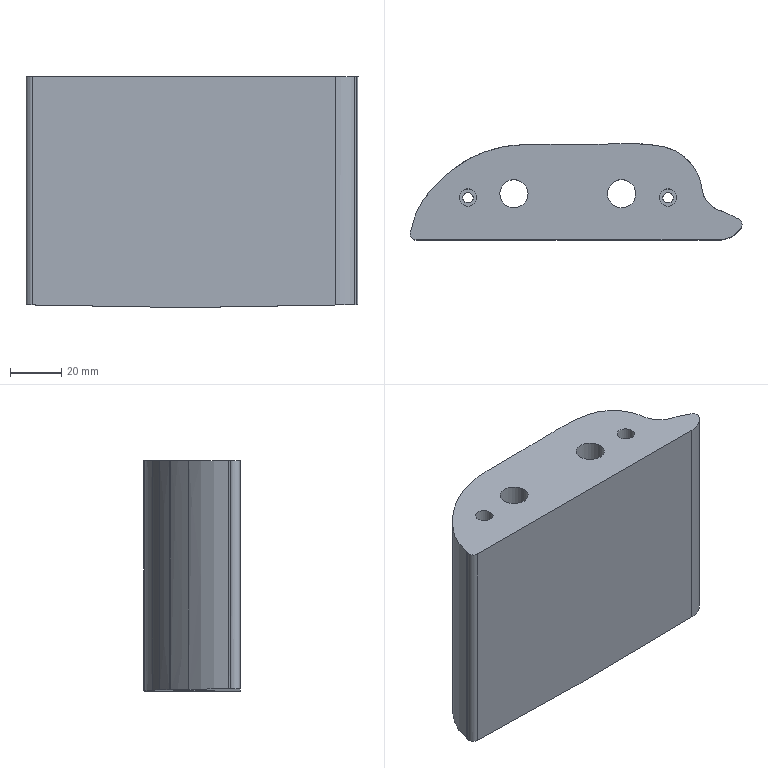Part | STEP file | gslz 2016.10.28-10_id2946_x_t | 1 solid | 41 faces | box 129.443 x 37.474 x 90 mm | volume 310631 mm3 | other 17 | cylinder 13 | plane 11 | commonest cylinder face diameters 5 x4 4.1 x2 6.8 x2 11 x2 17 x2 20 x1